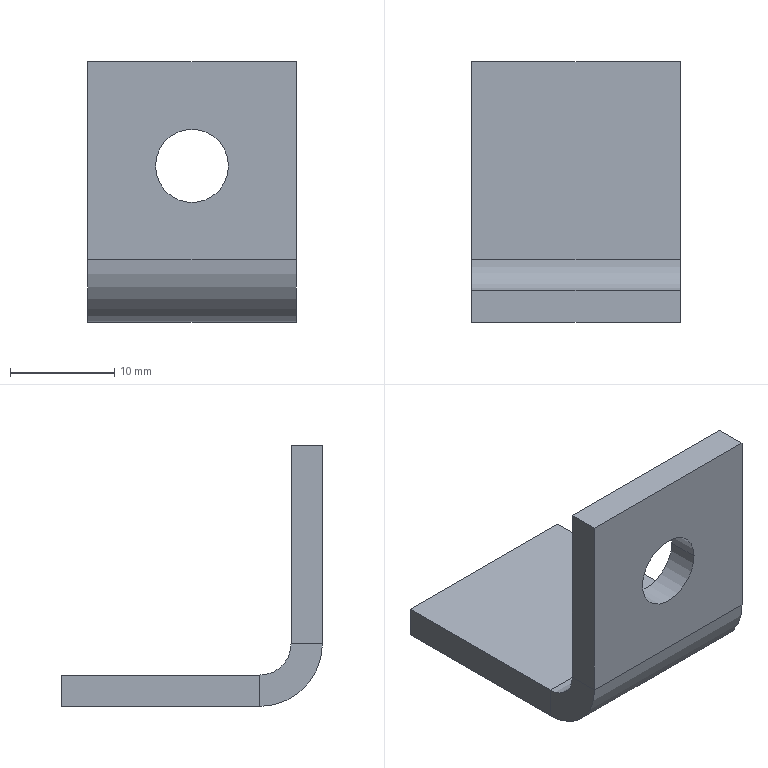Part | SolidWorks | 1 solid | 16 faces | box 20 x 25 x 25 mm | volume 2589 mm3 | plane 12 | cylinder 4 | commonest cylinder face diameters 7 x2 6 x1 12 x1
STEP:
#1=CARTESIAN_POINT('',(-13.5,0.,15.));
#2=VERTEX_POINT('',#1);
#3=CARTESIAN_POINT('',(-6.5,0.,15.));
#4=VERTEX_POINT('',#3);
#5=CARTESIAN_POINT('',(-10.,0.,15.));
#6=DIRECTION('',(0.,-1.,0.));
#7=DIRECTION('',(-1.,0.,0.));
#8=AXIS2_PLACEMENT_3D('',#5,#6,#7);
#9=CIRCLE('',#8,3.5);
#10=EDGE_CURVE('',#2,#4,#9,.T.);
#11=ORIENTED_EDGE('',*,*,#10,.T.);
#12=CARTESIAN_POINT('',(-6.5,3.,15.));
#13=VERTEX_POINT('',#12);
#14=CARTESIAN_POINT('',(-6.5,0.,15.));
#15=DIRECTION('',(0.,1.,0.));
#16=VECTOR('',#15,1000.);
#17=LINE('',#14,#16);
#18=EDGE_CURVE('',#4,#13,#17,.T.);
#19=ORIENTED_EDGE('',*,*,#18,.T.);
#20=CARTESIAN_POINT('',(-13.5,3.,15.));
#21=VERTEX_POINT('',#20);
#22=CARTESIAN_POINT('',(-10.,3.,15.));
#23=DIRECTION('',(0.,1.,0.));
#24=DIRECTION('',(1.,0.,0.));
#25=AXIS2_PLACEMENT_3D('',#22,#23,#24);
#26=CIRCLE('',#25,3.5);
#27=EDGE_CURVE('',#13,#21,#26,.T.);
#28=ORIENTED_EDGE('',*,*,#27,.T.);
#29=CARTESIAN_POINT('',(-13.5,0.,15.));
#30=DIRECTION('',(0.,1.,0.));
#31=VECTOR('',#30,1000.);
#32=LINE('',#29,#31);
#33=EDGE_CURVE('',#2,#21,#32,.T.);
#34=ORIENTED_EDGE('',*,*,#33,.F.);
#35=EDGE_LOOP('',(#11,#19,#28,#34));
#36=FACE_OUTER_BOUND('',#35,.T.);
#37=CARTESIAN_POINT('',(-10.,1.5,15.));
#38=DIRECTION('',(0.,-1.,0.));
#39=DIRECTION('',(1.,0.,0.));
#40=AXIS2_PLACEMENT_3D('',#37,#38,#39);
#41=CYLINDRICAL_SURFACE('',#40,3.5);
#42=ADVANCED_FACE('',(#36),#41,.F.);
#43=ORIENTED_EDGE('',*,*,#18,.F.);
#44=CARTESIAN_POINT('',(-10.,0.,15.));
#45=DIRECTION('',(0.,-1.,0.));
#46=DIRECTION('',(1.,0.,0.));
#47=AXIS2_PLACEMENT_3D('',#44,#45,#46);
#48=CIRCLE('',#47,3.5);
#49=EDGE_CURVE('',#4,#2,#48,.T.);
#50=ORIENTED_EDGE('',*,*,#49,.T.);
#51=ORIENTED_EDGE('',*,*,#33,.T.);
#52=CARTESIAN_POINT('',(-10.,3.,15.));
#53=DIRECTION('',(0.,1.,0.));
#54=DIRECTION('',(-1.,0.,0.));
#55=AXIS2_PLACEMENT_3D('',#52,#53,#54);
#56=CIRCLE('',#55,3.5);
#57=EDGE_CURVE('',#21,#13,#56,.T.);
#58=ORIENTED_EDGE('',*,*,#57,.T.);
#59=EDGE_LOOP('',(#43,#50,#51,#58));
#60=FACE_OUTER_BOUND('',#59,.T.);
#61=CARTESIAN_POINT('',(-10.,1.5,15.));
#62=DIRECTION('',(0.,-1.,0.));
#63=DIRECTION('',(1.,0.,0.));
#64=AXIS2_PLACEMENT_3D('',#61,#62,#63);
#65=CYLINDRICAL_SURFACE('',#64,3.5);
#66=ADVANCED_FACE('',(#60),#65,.F.);
#67=CARTESIAN_POINT('',(-20.,0.,25.));
#68=VERTEX_POINT('',#67);
#69=CARTESIAN_POINT('',(0.,0.,25.));
#70=VERTEX_POINT('',#69);
#71=CARTESIAN_POINT('',(-20.,0.,25.));
#72=DIRECTION('',(1.,0.,0.));
#73=VECTOR('',#72,1000.);
#74=LINE('',#71,#73);
#75=EDGE_CURVE('',#68,#70,#74,.T.);
#76=ORIENTED_EDGE('',*,*,#75,.T.);
#77=CARTESIAN_POINT('',(0.,3.,25.));
#78=VERTEX_POINT('',#77);
#79=CARTESIAN_POINT('',(0.,3.,25.));
#80=DIRECTION('',(0.,-1.,0.));
#81=VECTOR('',#80,1000.);
#82=LINE('',#79,#81);
#83=EDGE_CURVE('',#78,#70,#82,.T.);
#84=ORIENTED_EDGE('',*,*,#83,.F.);
#85=CARTESIAN_POINT('',(-20.,3.,25.));
#86=VERTEX_POINT('',#85);
#87=CARTESIAN_POINT('',(-20.,3.,25.));
#88=DIRECTION('',(1.,0.,0.));
#89=VECTOR('',#88,1000.);
#90=LINE('',#87,#89);
#91=EDGE_CURVE('',#86,#78,#90,.T.);
#92=ORIENTED_EDGE('',*,*,#91,.F.);
#93=CARTESIAN_POINT('',(-20.,3.,25.));
#94=DIRECTION('',(0.,-1.,0.));
#95=VECTOR('',#94,1000.);
#96=LINE('',#93,#95);
#97=EDGE_CURVE('',#86,#68,#96,.T.);
#98=ORIENTED_EDGE('',*,*,#97,.T.);
#99=EDGE_LOOP('',(#76,#84,#92,#98));
#100=FACE_OUTER_BOUND('',#99,.T.);
#101=CARTESIAN_POINT('',(0.,0.,25.));
#102=DIRECTION('',(0.,0.,1.));
#103=DIRECTION('',(1.,0.,0.));
#104=AXIS2_PLACEMENT_3D('',#101,#102,#103);
#105=PLANE('',#104);
#106=ADVANCED_FACE('',(#100),#105,.T.);
#107=CARTESIAN_POINT('',(-20.,25.,3.));
#108=VERTEX_POINT('',#107);
#109=CARTESIAN_POINT('',(0.,25.,3.));
#110=VERTEX_POINT('',#109);
#111=CARTESIAN_POINT('',(-20.,25.,3.));
#112=DIRECTION('',(1.,0.,0.));
#113=VECTOR('',#112,1000.);
#114=LINE('',#111,#113);
#115=EDGE_CURVE('',#108,#110,#114,.T.);
#116=ORIENTED_EDGE('',*,*,#115,.T.);
#117=CARTESIAN_POINT('',(0.,25.,0.));
#118=VERTEX_POINT('',#117);
#119=CARTESIAN_POINT('',(0.,25.,0.));
#120=DIRECTION('',(0.,0.,1.));
#121=VECTOR('',#120,1000.);
#122=LINE('',#119,#121);
#123=EDGE_CURVE('',#118,#110,#122,.T.);
#124=ORIENTED_EDGE('',*,*,#123,.F.);
#125=CARTESIAN_POINT('',(-20.,25.,0.));
#126=VERTEX_POINT('',#125);
#127=CARTESIAN_POINT('',(-20.,25.,0.));
#128=DIRECTION('',(1.,0.,0.));
#129=VECTOR('',#128,1000.);
#130=LINE('',#127,#129);
#131=EDGE_CURVE('',#126,#118,#130,.T.);
#132=ORIENTED_EDGE('',*,*,#131,.F.);
#133=CARTESIAN_POINT('',(-20.,25.,0.));
#134=DIRECTION('',(0.,0.,1.));
#135=VECTOR('',#134,1000.);
#136=LINE('',#133,#135);
#137=EDGE_CURVE('',#126,#108,#136,.T.);
#138=ORIENTED_EDGE('',*,*,#137,.T.);
#139=EDGE_LOOP('',(#116,#124,#132,#138));
#140=FACE_OUTER_BOUND('',#139,.T.);
#141=CARTESIAN_POINT('',(0.,25.,3.));
#142=DIRECTION('',(0.,1.,0.));
#143=DIRECTION('',(1.,0.,0.));
#144=AXIS2_PLACEMENT_3D('',#141,#142,#143);
#145=PLANE('',#144);
#146=ADVANCED_FACE('',(#140),#145,.T.);
#147=ORIENTED_EDGE('',*,*,#131,.T.);
#148=CARTESIAN_POINT('',(0.,6.,0.));
#149=VERTEX_POINT('',#148);
#150=CARTESIAN_POINT('',(0.,25.,0.));
#151=DIRECTION('',(0.,-1.,0.));
#152=VECTOR('',#151,1000.);
#153=LINE('',#150,#152);
#154=EDGE_CURVE('',#118,#149,#153,.T.);
#155=ORIENTED_EDGE('',*,*,#154,.T.);
#156=CARTESIAN_POINT('',(-20.,6.,0.));
#157=VERTEX_POINT('',#156);
#158=CARTESIAN_POINT('',(0.,6.,0.));
#159=DIRECTION('',(-1.,0.,0.));
#160=VECTOR('',#159,1000.);
#161=LINE('',#158,#160);
#162=EDGE_CURVE('',#149,#157,#161,.T.);
#163=ORIENTED_EDGE('',*,*,#162,.T.);
#164=CARTESIAN_POINT('',(-20.,6.,0.));
#165=DIRECTION('',(0.,1.,0.));
#166=VECTOR('',#165,1000.);
#167=LINE('',#164,#166);
#168=EDGE_CURVE('',#157,#126,#167,.T.);
#169=ORIENTED_EDGE('',*,*,#168,.T.);
#170=EDGE_LOOP('',(#147,#155,#163,#169));
#171=FACE_OUTER_BOUND('',#170,.T.);
#172=CARTESIAN_POINT('',(-10.,12.107,0.));
#173=DIRECTION('',(0.,0.,1.));
#174=DIRECTION('',(1.,0.,0.));
#175=AXIS2_PLACEMENT_3D('',#172,#173,#174);
#176=PLANE('',#175);
#177=ADVANCED_FACE('',(#171),#176,.F.);
#178=ORIENTED_EDGE('',*,*,#123,.T.);
#179=CARTESIAN_POINT('',(0.,6.,3.));
#180=VERTEX_POINT('',#179);
#181=CARTESIAN_POINT('',(0.,6.,3.));
#182=DIRECTION('',(0.,1.,0.));
#183=VECTOR('',#182,1000.);
#184=LINE('',#181,#183);
#185=EDGE_CURVE('',#180,#110,#184,.T.);
#186=ORIENTED_EDGE('',*,*,#185,.F.);
#187=CARTESIAN_POINT('',(0.,6.,0.));
#188=DIRECTION('',(0.,0.,1.));
#189=VECTOR('',#188,1000.);
#190=LINE('',#187,#189);
#191=EDGE_CURVE('',#149,#180,#190,.T.);
#192=ORIENTED_EDGE('',*,*,#191,.F.);
#193=ORIENTED_EDGE('',*,*,#154,.F.);
#194=EDGE_LOOP('',(#178,#186,#192,#193));
#195=FACE_OUTER_BOUND('',#194,.T.);
#196=CARTESIAN_POINT('',(0.,6.,3.));
#197=DIRECTION('',(1.,0.,0.));
#198=DIRECTION('',(0.,1.,0.));
#199=AXIS2_PLACEMENT_3D('',#196,#197,#198);
#200=PLANE('',#199);
#201=ADVANCED_FACE('',(#195),#200,.T.);
#202=ORIENTED_EDGE('',*,*,#115,.F.);
#203=CARTESIAN_POINT('',(-20.,6.,3.));
#204=VERTEX_POINT('',#203);
#205=CARTESIAN_POINT('',(-20.,6.,3.));
#206=DIRECTION('',(0.,1.,0.));
#207=VECTOR('',#206,1000.);
#208=LINE('',#205,#207);
#209=EDGE_CURVE('',#204,#108,#208,.T.);
#210=ORIENTED_EDGE('',*,*,#209,.F.);
#211=CARTESIAN_POINT('',(-20.,6.,3.));
#212=DIRECTION('',(1.,0.,0.));
#213=VECTOR('',#212,1000.);
#214=LINE('',#211,#213);
#215=EDGE_CURVE('',#204,#180,#214,.T.);
#216=ORIENTED_EDGE('',*,*,#215,.T.);
#217=ORIENTED_EDGE('',*,*,#185,.T.);
#218=EDGE_LOOP('',(#202,#210,#216,#217));
#219=FACE_OUTER_BOUND('',#218,.T.);
#220=CARTESIAN_POINT('',(-10.,12.107,3.));
#221=DIRECTION('',(0.,0.,1.));
#222=DIRECTION('',(1.,0.,0.));
#223=AXIS2_PLACEMENT_3D('',#220,#221,#222);
#224=PLANE('',#223);
#225=ADVANCED_FACE('',(#219),#224,.T.);
#226=ORIENTED_EDGE('',*,*,#137,.F.);
#227=ORIENTED_EDGE('',*,*,#168,.F.);
#228=CARTESIAN_POINT('',(-20.,6.,3.));
#229=DIRECTION('',(0.,0.,-1.));
#230=VECTOR('',#229,1000.);
#231=LINE('',#228,#230);
#232=EDGE_CURVE('',#204,#157,#231,.T.);
#233=ORIENTED_EDGE('',*,*,#232,.F.);
#234=ORIENTED_EDGE('',*,*,#209,.T.);
#235=EDGE_LOOP('',(#226,#227,#233,#234));
#236=FACE_OUTER_BOUND('',#235,.T.);
#237=CARTESIAN_POINT('',(-20.,6.,3.));
#238=DIRECTION('',(-1.,0.,0.));
#239=DIRECTION('',(0.,0.,1.));
#240=AXIS2_PLACEMENT_3D('',#237,#238,#239);
#241=PLANE('',#240);
#242=ADVANCED_FACE('',(#236),#241,.T.);
#243=CARTESIAN_POINT('',(-20.,0.,6.));
#244=VERTEX_POINT('',#243);
#245=CARTESIAN_POINT('',(-20.,3.,6.));
#246=VERTEX_POINT('',#245);
#247=CARTESIAN_POINT('',(-20.,0.,6.));
#248=DIRECTION('',(0.,1.,0.));
#249=VECTOR('',#248,1000.);
#250=LINE('',#247,#249);
#251=EDGE_CURVE('',#244,#246,#250,.T.);
#252=ORIENTED_EDGE('',*,*,#251,.T.);
#253=CARTESIAN_POINT('',(-20.,6.,6.));
#254=DIRECTION('',(-1.,0.,0.));
#255=DIRECTION('',(0.,0.,-1.));
#256=AXIS2_PLACEMENT_3D('',#253,#254,#255);
#257=CIRCLE('',#256,3.);
#258=EDGE_CURVE('',#204,#246,#257,.T.);
#259=ORIENTED_EDGE('',*,*,#258,.F.);
#260=ORIENTED_EDGE('',*,*,#232,.T.);
#261=CARTESIAN_POINT('',(-20.,6.,6.));
#262=DIRECTION('',(1.,0.,0.));
#263=DIRECTION('',(0.,-1.,0.));
#264=AXIS2_PLACEMENT_3D('',#261,#262,#263);
#265=CIRCLE('',#264,6.);
#266=EDGE_CURVE('',#244,#157,#265,.T.);
#267=ORIENTED_EDGE('',*,*,#266,.F.);
#268=EDGE_LOOP('',(#252,#259,#260,#267));
#269=FACE_OUTER_BOUND('',#268,.T.);
#270=CARTESIAN_POINT('',(-20.,6.,0.));
#271=DIRECTION('',(-1.,0.,0.));
#272=DIRECTION('',(0.,0.,1.));
#273=AXIS2_PLACEMENT_3D('',#270,#271,#272);
#274=PLANE('',#273);
#275=ADVANCED_FACE('',(#269),#274,.T.);
#276=CARTESIAN_POINT('',(0.,3.,6.));
#277=VERTEX_POINT('',#276);
#278=CARTESIAN_POINT('',(0.,3.,6.));
#279=DIRECTION('',(-1.,0.,0.));
#280=VECTOR('',#279,1000.);
#281=LINE('',#278,#280);
#282=EDGE_CURVE('',#277,#246,#281,.T.);
#283=ORIENTED_EDGE('',*,*,#282,.F.);
#284=CARTESIAN_POINT('',(0.,6.,6.));
#285=DIRECTION('',(1.,0.,0.));
#286=DIRECTION('',(0.,-1.,0.));
#287=AXIS2_PLACEMENT_3D('',#284,#285,#286);
#288=CIRCLE('',#287,3.);
#289=EDGE_CURVE('',#277,#180,#288,.T.);
#290=ORIENTED_EDGE('',*,*,#289,.T.);
#291=ORIENTED_EDGE('',*,*,#215,.F.);
#292=ORIENTED_EDGE('',*,*,#258,.T.);
#293=EDGE_LOOP('',(#283,#290,#291,#292));
#294=FACE_OUTER_BOUND('',#293,.T.);
#295=CARTESIAN_POINT('',(-10.,6.,6.));
#296=DIRECTION('',(1.,0.,0.));
#297=DIRECTION('',(0.,-1.,0.));
#298=AXIS2_PLACEMENT_3D('',#295,#296,#297);
#299=CYLINDRICAL_SURFACE('',#298,3.);
#300=ADVANCED_FACE('',(#294),#299,.F.);
#301=CARTESIAN_POINT('',(0.,0.,6.));
#302=VERTEX_POINT('',#301);
#303=CARTESIAN_POINT('',(0.,3.,6.));
#304=DIRECTION('',(0.,-1.,0.));
#305=VECTOR('',#304,1000.);
#306=LINE('',#303,#305);
#307=EDGE_CURVE('',#277,#302,#306,.T.);
#308=ORIENTED_EDGE('',*,*,#307,.T.);
#309=CARTESIAN_POINT('',(0.,6.,6.));
#310=DIRECTION('',(-1.,0.,0.));
#311=DIRECTION('',(0.,0.,-1.));
#312=AXIS2_PLACEMENT_3D('',#309,#310,#311);
#313=CIRCLE('',#312,6.);
#314=EDGE_CURVE('',#149,#302,#313,.T.);
#315=ORIENTED_EDGE('',*,*,#314,.F.);
#316=ORIENTED_EDGE('',*,*,#191,.T.);
#317=ORIENTED_EDGE('',*,*,#289,.F.);
#318=EDGE_LOOP('',(#308,#315,#316,#317));
#319=FACE_OUTER_BOUND('',#318,.T.);
#320=CARTESIAN_POINT('',(0.,6.,3.));
#321=DIRECTION('',(1.,0.,0.));
#322=DIRECTION('',(0.,1.,0.));
#323=AXIS2_PLACEMENT_3D('',#320,#321,#322);
#324=PLANE('',#323);
#325=ADVANCED_FACE('',(#319),#324,.T.);
#326=CARTESIAN_POINT('',(-20.,0.,6.));
#327=DIRECTION('',(1.,0.,0.));
#328=VECTOR('',#327,1000.);
#329=LINE('',#326,#328);
#330=EDGE_CURVE('',#244,#302,#329,.T.);
#331=ORIENTED_EDGE('',*,*,#330,.F.);
#332=ORIENTED_EDGE('',*,*,#266,.T.);
#333=ORIENTED_EDGE('',*,*,#162,.F.);
#334=ORIENTED_EDGE('',*,*,#314,.T.);
#335=EDGE_LOOP('',(#331,#332,#333,#334));
#336=FACE_OUTER_BOUND('',#335,.T.);
#337=CARTESIAN_POINT('',(-10.,6.,6.));
#338=DIRECTION('',(1.,0.,0.));
#339=DIRECTION('',(0.,-1.,0.));
#340=AXIS2_PLACEMENT_3D('',#337,#338,#339);
#341=CYLINDRICAL_SURFACE('',#340,6.);
#342=ADVANCED_FACE('',(#336),#341,.T.);
#343=ORIENTED_EDGE('',*,*,#10,.F.);
#344=ORIENTED_EDGE('',*,*,#49,.F.);
#345=EDGE_LOOP('',(#343,#344));
#346=FACE_BOUND('',#345,.T.);
#347=ORIENTED_EDGE('',*,*,#75,.F.);
#348=CARTESIAN_POINT('',(-20.,0.,6.));
#349=DIRECTION('',(0.,0.,1.));
#350=VECTOR('',#349,1000.);
#351=LINE('',#348,#350);
#352=EDGE_CURVE('',#244,#68,#351,.T.);
#353=ORIENTED_EDGE('',*,*,#352,.F.);
#354=ORIENTED_EDGE('',*,*,#330,.T.);
#355=CARTESIAN_POINT('',(0.,0.,25.));
#356=DIRECTION('',(0.,0.,-1.));
#357=VECTOR('',#356,1000.);
#358=LINE('',#355,#357);
#359=EDGE_CURVE('',#70,#302,#358,.T.);
#360=ORIENTED_EDGE('',*,*,#359,.F.);
#361=EDGE_LOOP('',(#347,#353,#354,#360));
#362=FACE_OUTER_BOUND('',#361,.T.);
#363=CARTESIAN_POINT('',(-10.,0.,12.5));
#364=DIRECTION('',(0.,1.,0.));
#365=DIRECTION('',(1.,0.,0.));
#366=AXIS2_PLACEMENT_3D('',#363,#364,#365);
#367=PLANE('',#366);
#368=ADVANCED_FACE('',(#346,#362),#367,.F.);
#369=ORIENTED_EDGE('',*,*,#97,.F.);
#370=CARTESIAN_POINT('',(-20.,3.,6.));
#371=DIRECTION('',(0.,0.,1.));
#372=VECTOR('',#371,1000.);
#373=LINE('',#370,#372);
#374=EDGE_CURVE('',#246,#86,#373,.T.);
#375=ORIENTED_EDGE('',*,*,#374,.F.);
#376=ORIENTED_EDGE('',*,*,#251,.F.);
#377=ORIENTED_EDGE('',*,*,#352,.T.);
#378=EDGE_LOOP('',(#369,#375,#376,#377));
#379=FACE_OUTER_BOUND('',#378,.T.);
#380=CARTESIAN_POINT('',(-20.,0.,25.));
#381=DIRECTION('',(-1.,0.,0.));
#382=DIRECTION('',(0.,0.,1.));
#383=AXIS2_PLACEMENT_3D('',#380,#381,#382);
#384=PLANE('',#383);
#385=ADVANCED_FACE('',(#379),#384,.T.);
#386=ORIENTED_EDGE('',*,*,#57,.F.);
#387=ORIENTED_EDGE('',*,*,#27,.F.);
#388=EDGE_LOOP('',(#386,#387));
#389=FACE_BOUND('',#388,.T.);
#390=ORIENTED_EDGE('',*,*,#91,.T.);
#391=CARTESIAN_POINT('',(0.,3.,25.));
#392=DIRECTION('',(0.,0.,-1.));
#393=VECTOR('',#392,1000.);
#394=LINE('',#391,#393);
#395=EDGE_CURVE('',#78,#277,#394,.T.);
#396=ORIENTED_EDGE('',*,*,#395,.T.);
#397=ORIENTED_EDGE('',*,*,#282,.T.);
#398=ORIENTED_EDGE('',*,*,#374,.T.);
#399=EDGE_LOOP('',(#390,#396,#397,#398));
#400=FACE_OUTER_BOUND('',#399,.T.);
#401=CARTESIAN_POINT('',(-10.,3.,12.5));
#402=DIRECTION('',(0.,1.,0.));
#403=DIRECTION('',(1.,0.,0.));
#404=AXIS2_PLACEMENT_3D('',#401,#402,#403);
#405=PLANE('',#404);
#406=ADVANCED_FACE('',(#389,#400),#405,.T.);
#407=ORIENTED_EDGE('',*,*,#83,.T.);
#408=ORIENTED_EDGE('',*,*,#359,.T.);
#409=ORIENTED_EDGE('',*,*,#307,.F.);
#410=ORIENTED_EDGE('',*,*,#395,.F.);
#411=EDGE_LOOP('',(#407,#408,#409,#410));
#412=FACE_OUTER_BOUND('',#411,.T.);
#413=CARTESIAN_POINT('',(0.,0.,0.));
#414=DIRECTION('',(1.,0.,0.));
#415=DIRECTION('',(0.,1.,0.));
#416=AXIS2_PLACEMENT_3D('',#413,#414,#415);
#417=PLANE('',#416);
#418=ADVANCED_FACE('',(#412),#417,.T.);
#419=CLOSED_SHELL('',(#42,#66,#106,#146,#177,#201,#225,#242,#275,#300,#325,#342,#368,#385,#406,#418));
#420=MANIFOLD_SOLID_BREP('',#419);
#421=CARTESIAN_POINT('',(0.,0.,0.));
#422=DIRECTION('',(0.,0.,1.));
#423=DIRECTION('',(1.,0.,0.));
#424=AXIS2_PLACEMENT_3D('',#421,#422,#423);
#425=(LENGTH_UNIT()NAMED_UNIT(*)SI_UNIT(.MILLI.,.METRE.));
#426=UNCERTAINTY_MEASURE_WITH_UNIT(LENGTH_MEASURE(0.00001),#425,'','');
#427=(NAMED_UNIT(*)PLANE_ANGLE_UNIT()SI_UNIT($,.RADIAN.));
#428=(NAMED_UNIT(*)SI_UNIT($,.STERADIAN.)SOLID_ANGLE_UNIT());
#429=(GEOMETRIC_REPRESENTATION_CONTEXT(3)GLOBAL_UNCERTAINTY_ASSIGNED_CONTEXT((#426))GLOBAL_UNIT_ASSIGNED_CONTEXT((#425,#427,#428))REPRESENTATION_CONTEXT('',''));
#430=ADVANCED_BREP_SHAPE_REPRESENTATION('',(#420,#424),#429);